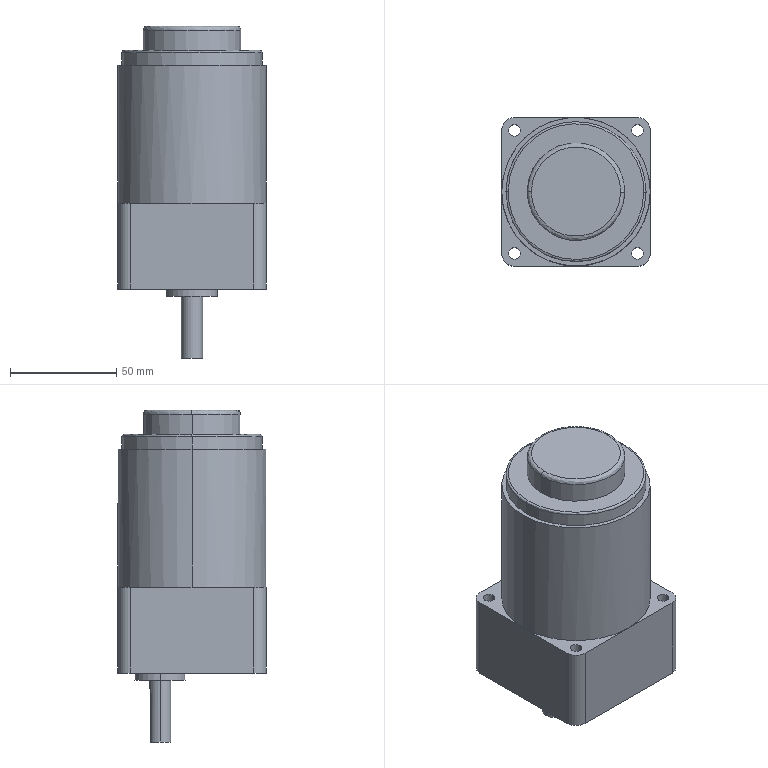Part | STEP file | 101-03-0011 | 1 solid | 47 faces | box 70 x 70 x 156.5 mm | volume 487470 mm3 | cylinder 24 | plane 19 | spline 4 | commonest cylinder face diameters 5.5 x8 12 x4 10 x2 24 x2 46 x2 62 x2